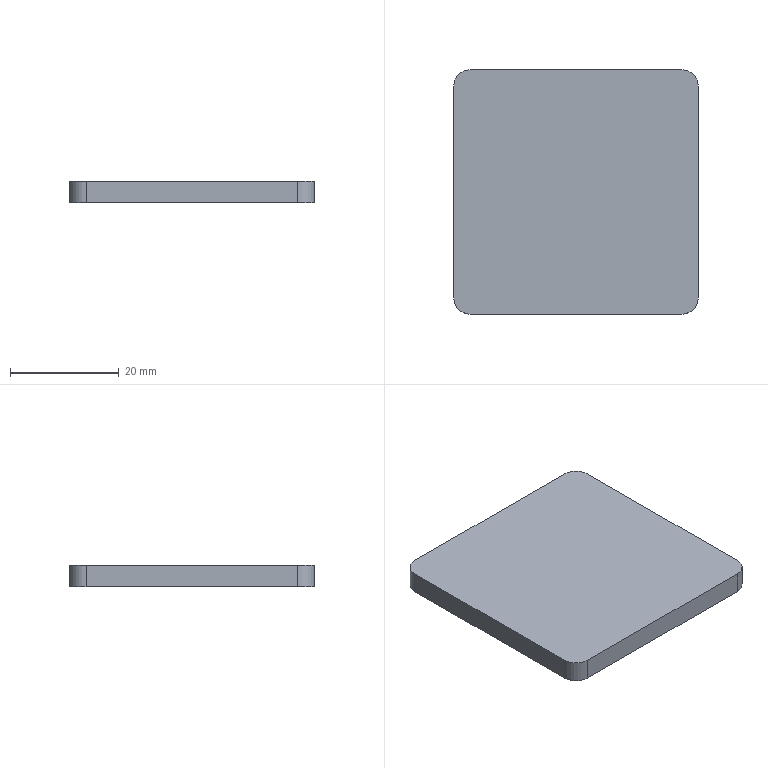Part | STEP file | 1 solid | 10 faces | box 45 x 45 x 4 mm | volume 8069 mm3 | plane 6 | cylinder 4 | commonest cylinder face diameters 6 x4
STEP:
#1=CARTESIAN_POINT('',(0.,0.,0.));
#2=DIRECTION('',(0.,0.,1.));
#3=DIRECTION('',(1.,0.,0.));
#4=AXIS2_PLACEMENT_3D('',#1,#2,#3);
#5=CARTESIAN_POINT('',(-527.5,-80.5,0.));
#6=VERTEX_POINT('',#5);
#7=CARTESIAN_POINT('',(-530.5,-77.5,0.));
#8=VERTEX_POINT('',#7);
#9=CARTESIAN_POINT('',(-530.5,-80.5,0.));
#10=DIRECTION('',(0.,0.,1.));
#11=DIRECTION('',(-1.,0.,0.));
#12=AXIS2_PLACEMENT_3D('',#9,#10,#11);
#13=CIRCLE('',#12,3.);
#14=CARTESIAN_POINT('',(-530.5,-80.5,0.));
#15=DIRECTION('',(0.,0.,-1.));
#16=DIRECTION('',(-1.,0.,0.));
#17=AXIS2_PLACEMENT_3D('',#14,#15,#16);
#18=PLANE('',#17);
#19=CARTESIAN_POINT('',(3.,0.));
#20=CARTESIAN_POINT('',(3.,-5.196));
#21=CARTESIAN_POINT('',(-1.5,-2.598));
#22=CARTESIAN_POINT('',(-6.,0.));
#23=CARTESIAN_POINT('',(-1.5,2.598));
#24=CARTESIAN_POINT('',(3.,5.196));
#25=CARTESIAN_POINT('',(3.,0.));
#26=(BOUNDED_CURVE()B_SPLINE_CURVE(2,(#19,#20,#21,#22,#23,#24,#25),.UNSPECIFIED.,.T.,.F.)B_SPLINE_CURVE_WITH_KNOTS((1,2,2,2,2,1),(-2.094,0.,2.094,4.189,6.283,8.378),.UNSPECIFIED.)CURVE()GEOMETRIC_REPRESENTATION_ITEM()RATIONAL_B_SPLINE_CURVE((1.,0.5,1.,0.5,1.,0.5,1.))REPRESENTATION_ITEM(''));
#27=(GEOMETRIC_REPRESENTATION_CONTEXT(2)PARAMETRIC_REPRESENTATION_CONTEXT()REPRESENTATION_CONTEXT('',''));
#28=DEFINITIONAL_REPRESENTATION('',(#26),#27);
#29=PCURVE('',#18,#28);
#30=CARTESIAN_POINT('',(-530.5,-80.5,4.));
#31=DIRECTION('',(0.,0.,-1.));
#32=DIRECTION('',(-1.,0.,0.));
#33=AXIS2_PLACEMENT_3D('',#30,#31,#32);
#34=CYLINDRICAL_SURFACE('',#33,3.);
#35=CARTESIAN_POINT('',(6.283,4.));
#36=DIRECTION('',(-1.,0.));
#37=VECTOR('',#36,1.);
#38=LINE('',#35,#37);
#39=(GEOMETRIC_REPRESENTATION_CONTEXT(2)PARAMETRIC_REPRESENTATION_CONTEXT()REPRESENTATION_CONTEXT('',''));
#40=DEFINITIONAL_REPRESENTATION('',(#38),#39);
#41=PCURVE('',#34,#40);
#42=SURFACE_CURVE('',#13,(#29,#41),.PCURVE_S1.);
#43=EDGE_CURVE('',#6,#8,#42,.T.);
#44=ORIENTED_EDGE('',*,*,#43,.F.);
#45=CARTESIAN_POINT('',(-527.5,-119.5,0.));
#46=VERTEX_POINT('',#45);
#47=CARTESIAN_POINT('',(-527.5,-80.5,0.));
#48=DIRECTION('',(0.,1.,0.));
#49=VECTOR('',#48,1.);
#50=LINE('',#47,#49);
#51=CARTESIAN_POINT('',(-3.,0.));
#52=DIRECTION('',(0.,1.));
#53=VECTOR('',#52,1.);
#54=LINE('',#51,#53);
#55=(GEOMETRIC_REPRESENTATION_CONTEXT(2)PARAMETRIC_REPRESENTATION_CONTEXT()REPRESENTATION_CONTEXT('',''));
#56=DEFINITIONAL_REPRESENTATION('',(#54),#55);
#57=PCURVE('',#18,#56);
#58=CARTESIAN_POINT('',(-527.5,-80.5,4.));
#59=DIRECTION('',(-1.,0.,0.));
#60=DIRECTION('',(0.,0.,1.));
#61=AXIS2_PLACEMENT_3D('',#58,#59,#60);
#62=PLANE('',#61);
#63=CARTESIAN_POINT('',(-4.,0.));
#64=DIRECTION('',(0.,1.));
#65=VECTOR('',#64,1.);
#66=LINE('',#63,#65);
#67=(GEOMETRIC_REPRESENTATION_CONTEXT(2)PARAMETRIC_REPRESENTATION_CONTEXT()REPRESENTATION_CONTEXT('',''));
#68=DEFINITIONAL_REPRESENTATION('',(#66),#67);
#69=PCURVE('',#62,#68);
#70=SURFACE_CURVE('',#50,(#57,#69),.PCURVE_S1.);
#71=EDGE_CURVE('',#46,#6,#70,.T.);
#72=ORIENTED_EDGE('',*,*,#71,.F.);
#73=CARTESIAN_POINT('',(-530.5,-122.5,0.));
#74=VERTEX_POINT('',#73);
#75=CARTESIAN_POINT('',(-530.5,-119.5,0.));
#76=DIRECTION('',(0.,0.,1.));
#77=DIRECTION('',(-1.,0.,0.));
#78=AXIS2_PLACEMENT_3D('',#75,#76,#77);
#79=CIRCLE('',#78,3.);
#80=CARTESIAN_POINT('',(3.,-39.));
#81=CARTESIAN_POINT('',(3.,-44.196));
#82=CARTESIAN_POINT('',(-1.5,-41.598));
#83=CARTESIAN_POINT('',(-6.,-39.));
#84=CARTESIAN_POINT('',(-1.5,-36.402));
#85=CARTESIAN_POINT('',(3.,-33.804));
#86=CARTESIAN_POINT('',(3.,-39.));
#87=(BOUNDED_CURVE()B_SPLINE_CURVE(2,(#80,#81,#82,#83,#84,#85,#86),.UNSPECIFIED.,.T.,.F.)B_SPLINE_CURVE_WITH_KNOTS((1,2,2,2,2,1),(-2.094,0.,2.094,4.189,6.283,8.378),.UNSPECIFIED.)CURVE()GEOMETRIC_REPRESENTATION_ITEM()RATIONAL_B_SPLINE_CURVE((1.,0.5,1.,0.5,1.,0.5,1.))REPRESENTATION_ITEM(''));
#88=(GEOMETRIC_REPRESENTATION_CONTEXT(2)PARAMETRIC_REPRESENTATION_CONTEXT()REPRESENTATION_CONTEXT('',''));
#89=DEFINITIONAL_REPRESENTATION('',(#87),#88);
#90=PCURVE('',#18,#89);
#91=CARTESIAN_POINT('',(-530.5,-119.5,4.));
#92=DIRECTION('',(0.,0.,-1.));
#93=DIRECTION('',(-1.,0.,0.));
#94=AXIS2_PLACEMENT_3D('',#91,#92,#93);
#95=CYLINDRICAL_SURFACE('',#94,3.);
#96=CARTESIAN_POINT('',(6.283,4.));
#97=DIRECTION('',(-1.,0.));
#98=VECTOR('',#97,1.);
#99=LINE('',#96,#98);
#100=(GEOMETRIC_REPRESENTATION_CONTEXT(2)PARAMETRIC_REPRESENTATION_CONTEXT()REPRESENTATION_CONTEXT('',''));
#101=DEFINITIONAL_REPRESENTATION('',(#99),#100);
#102=PCURVE('',#95,#101);
#103=SURFACE_CURVE('',#79,(#90,#102),.PCURVE_S1.);
#104=EDGE_CURVE('',#74,#46,#103,.T.);
#105=ORIENTED_EDGE('',*,*,#104,.F.);
#106=CARTESIAN_POINT('',(-569.5,-122.5,0.));
#107=VERTEX_POINT('',#106);
#108=CARTESIAN_POINT('',(-530.5,-122.5,0.));
#109=DIRECTION('',(1.,0.,0.));
#110=VECTOR('',#109,1.);
#111=LINE('',#108,#110);
#112=CARTESIAN_POINT('',(0.,-42.));
#113=DIRECTION('',(-1.,0.));
#114=VECTOR('',#113,1.);
#115=LINE('',#112,#114);
#116=(GEOMETRIC_REPRESENTATION_CONTEXT(2)PARAMETRIC_REPRESENTATION_CONTEXT()REPRESENTATION_CONTEXT('',''));
#117=DEFINITIONAL_REPRESENTATION('',(#115),#116);
#118=PCURVE('',#18,#117);
#119=CARTESIAN_POINT('',(-530.5,-122.5,4.));
#120=DIRECTION('',(0.,1.,0.));
#121=DIRECTION('',(1.,0.,0.));
#122=AXIS2_PLACEMENT_3D('',#119,#120,#121);
#123=PLANE('',#122);
#124=CARTESIAN_POINT('',(0.,4.));
#125=DIRECTION('',(1.,0.));
#126=VECTOR('',#125,1.);
#127=LINE('',#124,#126);
#128=(GEOMETRIC_REPRESENTATION_CONTEXT(2)PARAMETRIC_REPRESENTATION_CONTEXT()REPRESENTATION_CONTEXT('',''));
#129=DEFINITIONAL_REPRESENTATION('',(#127),#128);
#130=PCURVE('',#123,#129);
#131=SURFACE_CURVE('',#111,(#118,#130),.PCURVE_S1.);
#132=EDGE_CURVE('',#107,#74,#131,.T.);
#133=ORIENTED_EDGE('',*,*,#132,.F.);
#134=CARTESIAN_POINT('',(-572.5,-119.5,0.));
#135=VERTEX_POINT('',#134);
#136=CARTESIAN_POINT('',(-569.5,-119.5,0.));
#137=DIRECTION('',(0.,0.,1.));
#138=DIRECTION('',(-1.,0.,0.));
#139=AXIS2_PLACEMENT_3D('',#136,#137,#138);
#140=CIRCLE('',#139,3.);
#141=CARTESIAN_POINT('',(42.,-39.));
#142=CARTESIAN_POINT('',(42.,-44.196));
#143=CARTESIAN_POINT('',(37.5,-41.598));
#144=CARTESIAN_POINT('',(33.,-39.));
#145=CARTESIAN_POINT('',(37.5,-36.402));
#146=CARTESIAN_POINT('',(42.,-33.804));
#147=CARTESIAN_POINT('',(42.,-39.));
#148=(BOUNDED_CURVE()B_SPLINE_CURVE(2,(#141,#142,#143,#144,#145,#146,#147),.UNSPECIFIED.,.T.,.F.)B_SPLINE_CURVE_WITH_KNOTS((1,2,2,2,2,1),(-2.094,0.,2.094,4.189,6.283,8.378),.UNSPECIFIED.)CURVE()GEOMETRIC_REPRESENTATION_ITEM()RATIONAL_B_SPLINE_CURVE((1.,0.5,1.,0.5,1.,0.5,1.))REPRESENTATION_ITEM(''));
#149=(GEOMETRIC_REPRESENTATION_CONTEXT(2)PARAMETRIC_REPRESENTATION_CONTEXT()REPRESENTATION_CONTEXT('',''));
#150=DEFINITIONAL_REPRESENTATION('',(#148),#149);
#151=PCURVE('',#18,#150);
#152=CARTESIAN_POINT('',(-569.5,-119.5,4.));
#153=DIRECTION('',(0.,0.,-1.));
#154=DIRECTION('',(-1.,0.,0.));
#155=AXIS2_PLACEMENT_3D('',#152,#153,#154);
#156=CYLINDRICAL_SURFACE('',#155,3.);
#157=CARTESIAN_POINT('',(6.283,4.));
#158=DIRECTION('',(-1.,0.));
#159=VECTOR('',#158,1.);
#160=LINE('',#157,#159);
#161=(GEOMETRIC_REPRESENTATION_CONTEXT(2)PARAMETRIC_REPRESENTATION_CONTEXT()REPRESENTATION_CONTEXT('',''));
#162=DEFINITIONAL_REPRESENTATION('',(#160),#161);
#163=PCURVE('',#156,#162);
#164=SURFACE_CURVE('',#140,(#151,#163),.PCURVE_S1.);
#165=EDGE_CURVE('',#135,#107,#164,.T.);
#166=ORIENTED_EDGE('',*,*,#165,.F.);
#167=CARTESIAN_POINT('',(-572.5,-80.5,0.));
#168=VERTEX_POINT('',#167);
#169=CARTESIAN_POINT('',(-572.5,-80.5,0.));
#170=DIRECTION('',(0.,-1.,0.));
#171=VECTOR('',#170,1.);
#172=LINE('',#169,#171);
#173=CARTESIAN_POINT('',(42.,0.));
#174=DIRECTION('',(0.,-1.));
#175=VECTOR('',#174,1.);
#176=LINE('',#173,#175);
#177=(GEOMETRIC_REPRESENTATION_CONTEXT(2)PARAMETRIC_REPRESENTATION_CONTEXT()REPRESENTATION_CONTEXT('',''));
#178=DEFINITIONAL_REPRESENTATION('',(#176),#177);
#179=PCURVE('',#18,#178);
#180=CARTESIAN_POINT('',(-572.5,-80.5,4.));
#181=DIRECTION('',(1.,0.,0.));
#182=DIRECTION('',(0.,0.,1.));
#183=AXIS2_PLACEMENT_3D('',#180,#181,#182);
#184=PLANE('',#183);
#185=CARTESIAN_POINT('',(-4.,0.));
#186=DIRECTION('',(0.,1.));
#187=VECTOR('',#186,1.);
#188=LINE('',#185,#187);
#189=(GEOMETRIC_REPRESENTATION_CONTEXT(2)PARAMETRIC_REPRESENTATION_CONTEXT()REPRESENTATION_CONTEXT('',''));
#190=DEFINITIONAL_REPRESENTATION('',(#188),#189);
#191=PCURVE('',#184,#190);
#192=SURFACE_CURVE('',#172,(#179,#191),.PCURVE_S1.);
#193=EDGE_CURVE('',#168,#135,#192,.T.);
#194=ORIENTED_EDGE('',*,*,#193,.F.);
#195=CARTESIAN_POINT('',(-569.5,-77.5,0.));
#196=VERTEX_POINT('',#195);
#197=CARTESIAN_POINT('',(-569.5,-80.5,0.));
#198=DIRECTION('',(0.,0.,1.));
#199=DIRECTION('',(1.,0.,0.));
#200=AXIS2_PLACEMENT_3D('',#197,#198,#199);
#201=CIRCLE('',#200,3.);
#202=CARTESIAN_POINT('',(36.,0.));
#203=CARTESIAN_POINT('',(36.,5.196));
#204=CARTESIAN_POINT('',(40.5,2.598));
#205=CARTESIAN_POINT('',(45.,0.));
#206=CARTESIAN_POINT('',(40.5,-2.598));
#207=CARTESIAN_POINT('',(36.,-5.196));
#208=CARTESIAN_POINT('',(36.,0.));
#209=(BOUNDED_CURVE()B_SPLINE_CURVE(2,(#202,#203,#204,#205,#206,#207,#208),.UNSPECIFIED.,.T.,.F.)B_SPLINE_CURVE_WITH_KNOTS((1,2,2,2,2,1),(-2.094,0.,2.094,4.189,6.283,8.378),.UNSPECIFIED.)CURVE()GEOMETRIC_REPRESENTATION_ITEM()RATIONAL_B_SPLINE_CURVE((1.,0.5,1.,0.5,1.,0.5,1.))REPRESENTATION_ITEM(''));
#210=(GEOMETRIC_REPRESENTATION_CONTEXT(2)PARAMETRIC_REPRESENTATION_CONTEXT()REPRESENTATION_CONTEXT('',''));
#211=DEFINITIONAL_REPRESENTATION('',(#209),#210);
#212=PCURVE('',#18,#211);
#213=CARTESIAN_POINT('',(-569.5,-80.5,4.));
#214=DIRECTION('',(0.,0.,-1.));
#215=DIRECTION('',(-1.,0.,0.));
#216=AXIS2_PLACEMENT_3D('',#213,#214,#215);
#217=CYLINDRICAL_SURFACE('',#216,3.);
#218=CARTESIAN_POINT('',(3.142,4.));
#219=DIRECTION('',(-1.,0.));
#220=VECTOR('',#219,1.);
#221=LINE('',#218,#220);
#222=(GEOMETRIC_REPRESENTATION_CONTEXT(2)PARAMETRIC_REPRESENTATION_CONTEXT()REPRESENTATION_CONTEXT('',''));
#223=DEFINITIONAL_REPRESENTATION('',(#221),#222);
#224=PCURVE('',#217,#223);
#225=SURFACE_CURVE('',#201,(#212,#224),.PCURVE_S1.);
#226=EDGE_CURVE('',#196,#168,#225,.T.);
#227=ORIENTED_EDGE('',*,*,#226,.F.);
#228=CARTESIAN_POINT('',(-530.5,-77.5,0.));
#229=DIRECTION('',(-1.,0.,0.));
#230=VECTOR('',#229,1.);
#231=LINE('',#228,#230);
#232=CARTESIAN_POINT('',(0.,3.));
#233=DIRECTION('',(1.,0.));
#234=VECTOR('',#233,1.);
#235=LINE('',#232,#234);
#236=(GEOMETRIC_REPRESENTATION_CONTEXT(2)PARAMETRIC_REPRESENTATION_CONTEXT()REPRESENTATION_CONTEXT('',''));
#237=DEFINITIONAL_REPRESENTATION('',(#235),#236);
#238=PCURVE('',#18,#237);
#239=CARTESIAN_POINT('',(-530.5,-77.5,4.));
#240=DIRECTION('',(0.,-1.,0.));
#241=DIRECTION('',(0.,0.,-1.));
#242=AXIS2_PLACEMENT_3D('',#239,#240,#241);
#243=PLANE('',#242);
#244=CARTESIAN_POINT('',(4.,0.));
#245=DIRECTION('',(0.,-1.));
#246=VECTOR('',#245,1.);
#247=LINE('',#244,#246);
#248=(GEOMETRIC_REPRESENTATION_CONTEXT(2)PARAMETRIC_REPRESENTATION_CONTEXT()REPRESENTATION_CONTEXT('',''));
#249=DEFINITIONAL_REPRESENTATION('',(#247),#248);
#250=PCURVE('',#243,#249);
#251=SURFACE_CURVE('',#231,(#238,#250),.PCURVE_S1.);
#252=EDGE_CURVE('',#8,#196,#251,.T.);
#253=ORIENTED_EDGE('',*,*,#252,.F.);
#254=EDGE_LOOP('',(#44,#72,#105,#133,#166,#194,#227,#253));
#255=FACE_BOUND('',#254,.T.);
#256=ADVANCED_FACE('',(#255),#18,.T.);
#257=CARTESIAN_POINT('',(-527.5,-80.5,4.));
#258=VERTEX_POINT('',#257);
#259=CARTESIAN_POINT('',(-530.5,-77.5,4.));
#260=VERTEX_POINT('',#259);
#261=CARTESIAN_POINT('',(-530.5,-80.5,4.));
#262=DIRECTION('',(0.,0.,1.));
#263=DIRECTION('',(-1.,0.,0.));
#264=AXIS2_PLACEMENT_3D('',#261,#262,#263);
#265=CIRCLE('',#264,3.);
#266=CARTESIAN_POINT('',(-530.5,-80.5,4.));
#267=DIRECTION('',(0.,0.,-1.));
#268=DIRECTION('',(-1.,0.,0.));
#269=AXIS2_PLACEMENT_3D('',#266,#267,#268);
#270=PLANE('',#269);
#271=CARTESIAN_POINT('',(3.,0.));
#272=CARTESIAN_POINT('',(3.,-5.196));
#273=CARTESIAN_POINT('',(-1.5,-2.598));
#274=CARTESIAN_POINT('',(-6.,0.));
#275=CARTESIAN_POINT('',(-1.5,2.598));
#276=CARTESIAN_POINT('',(3.,5.196));
#277=CARTESIAN_POINT('',(3.,0.));
#278=(BOUNDED_CURVE()B_SPLINE_CURVE(2,(#271,#272,#273,#274,#275,#276,#277),.UNSPECIFIED.,.T.,.F.)B_SPLINE_CURVE_WITH_KNOTS((1,2,2,2,2,1),(-2.094,0.,2.094,4.189,6.283,8.378),.UNSPECIFIED.)CURVE()GEOMETRIC_REPRESENTATION_ITEM()RATIONAL_B_SPLINE_CURVE((1.,0.5,1.,0.5,1.,0.5,1.))REPRESENTATION_ITEM(''));
#279=(GEOMETRIC_REPRESENTATION_CONTEXT(2)PARAMETRIC_REPRESENTATION_CONTEXT()REPRESENTATION_CONTEXT('',''));
#280=DEFINITIONAL_REPRESENTATION('',(#278),#279);
#281=PCURVE('',#270,#280);
#282=CARTESIAN_POINT('',(6.283,0.));
#283=DIRECTION('',(-1.,0.));
#284=VECTOR('',#283,1.);
#285=LINE('',#282,#284);
#286=(GEOMETRIC_REPRESENTATION_CONTEXT(2)PARAMETRIC_REPRESENTATION_CONTEXT()REPRESENTATION_CONTEXT('',''));
#287=DEFINITIONAL_REPRESENTATION('',(#285),#286);
#288=PCURVE('',#34,#287);
#289=SURFACE_CURVE('',#265,(#281,#288),.PCURVE_S1.);
#290=EDGE_CURVE('',#258,#260,#289,.T.);
#291=ORIENTED_EDGE('',*,*,#290,.T.);
#292=CARTESIAN_POINT('',(-569.5,-77.5,4.));
#293=VERTEX_POINT('',#292);
#294=CARTESIAN_POINT('',(-530.5,-77.5,4.));
#295=DIRECTION('',(-1.,0.,0.));
#296=VECTOR('',#295,1.);
#297=LINE('',#294,#296);
#298=CARTESIAN_POINT('',(0.,3.));
#299=DIRECTION('',(1.,0.));
#300=VECTOR('',#299,1.);
#301=LINE('',#298,#300);
#302=(GEOMETRIC_REPRESENTATION_CONTEXT(2)PARAMETRIC_REPRESENTATION_CONTEXT()REPRESENTATION_CONTEXT('',''));
#303=DEFINITIONAL_REPRESENTATION('',(#301),#302);
#304=PCURVE('',#270,#303);
#305=CARTESIAN_POINT('',(0.,0.));
#306=DIRECTION('',(0.,-1.));
#307=VECTOR('',#306,1.);
#308=LINE('',#305,#307);
#309=(GEOMETRIC_REPRESENTATION_CONTEXT(2)PARAMETRIC_REPRESENTATION_CONTEXT()REPRESENTATION_CONTEXT('',''));
#310=DEFINITIONAL_REPRESENTATION('',(#308),#309);
#311=PCURVE('',#243,#310);
#312=SURFACE_CURVE('',#297,(#304,#311),.PCURVE_S1.);
#313=EDGE_CURVE('',#260,#293,#312,.T.);
#314=ORIENTED_EDGE('',*,*,#313,.T.);
#315=CARTESIAN_POINT('',(-572.5,-80.5,4.));
#316=VERTEX_POINT('',#315);
#317=CARTESIAN_POINT('',(-569.5,-80.5,4.));
#318=DIRECTION('',(0.,0.,1.));
#319=DIRECTION('',(1.,0.,0.));
#320=AXIS2_PLACEMENT_3D('',#317,#318,#319);
#321=CIRCLE('',#320,3.);
#322=CARTESIAN_POINT('',(36.,0.));
#323=CARTESIAN_POINT('',(36.,5.196));
#324=CARTESIAN_POINT('',(40.5,2.598));
#325=CARTESIAN_POINT('',(45.,0.));
#326=CARTESIAN_POINT('',(40.5,-2.598));
#327=CARTESIAN_POINT('',(36.,-5.196));
#328=CARTESIAN_POINT('',(36.,0.));
#329=(BOUNDED_CURVE()B_SPLINE_CURVE(2,(#322,#323,#324,#325,#326,#327,#328),.UNSPECIFIED.,.T.,.F.)B_SPLINE_CURVE_WITH_KNOTS((1,2,2,2,2,1),(-2.094,0.,2.094,4.189,6.283,8.378),.UNSPECIFIED.)CURVE()GEOMETRIC_REPRESENTATION_ITEM()RATIONAL_B_SPLINE_CURVE((1.,0.5,1.,0.5,1.,0.5,1.))REPRESENTATION_ITEM(''));
#330=(GEOMETRIC_REPRESENTATION_CONTEXT(2)PARAMETRIC_REPRESENTATION_CONTEXT()REPRESENTATION_CONTEXT('',''));
#331=DEFINITIONAL_REPRESENTATION('',(#329),#330);
#332=PCURVE('',#270,#331);
#333=CARTESIAN_POINT('',(3.142,0.));
#334=DIRECTION('',(-1.,0.));
#335=VECTOR('',#334,1.);
#336=LINE('',#333,#335);
#337=(GEOMETRIC_REPRESENTATION_CONTEXT(2)PARAMETRIC_REPRESENTATION_CONTEXT()REPRESENTATION_CONTEXT('',''));
#338=DEFINITIONAL_REPRESENTATION('',(#336),#337);
#339=PCURVE('',#217,#338);
#340=SURFACE_CURVE('',#321,(#332,#339),.PCURVE_S1.);
#341=EDGE_CURVE('',#293,#316,#340,.T.);
#342=ORIENTED_EDGE('',*,*,#341,.T.);
#343=CARTESIAN_POINT('',(-572.5,-119.5,4.));
#344=VERTEX_POINT('',#343);
#345=CARTESIAN_POINT('',(-572.5,-80.5,4.));
#346=DIRECTION('',(0.,-1.,0.));
#347=VECTOR('',#346,1.);
#348=LINE('',#345,#347);
#349=CARTESIAN_POINT('',(42.,0.));
#350=DIRECTION('',(0.,-1.));
#351=VECTOR('',#350,1.);
#352=LINE('',#349,#351);
#353=(GEOMETRIC_REPRESENTATION_CONTEXT(2)PARAMETRIC_REPRESENTATION_CONTEXT()REPRESENTATION_CONTEXT('',''));
#354=DEFINITIONAL_REPRESENTATION('',(#352),#353);
#355=PCURVE('',#270,#354);
#356=CARTESIAN_POINT('',(0.,0.));
#357=DIRECTION('',(0.,1.));
#358=VECTOR('',#357,1.);
#359=LINE('',#356,#358);
#360=(GEOMETRIC_REPRESENTATION_CONTEXT(2)PARAMETRIC_REPRESENTATION_CONTEXT()REPRESENTATION_CONTEXT('',''));
#361=DEFINITIONAL_REPRESENTATION('',(#359),#360);
#362=PCURVE('',#184,#361);
#363=SURFACE_CURVE('',#348,(#355,#362),.PCURVE_S1.);
#364=EDGE_CURVE('',#316,#344,#363,.T.);
#365=ORIENTED_EDGE('',*,*,#364,.T.);
#366=CARTESIAN_POINT('',(-569.5,-122.5,4.));
#367=VERTEX_POINT('',#366);
#368=CARTESIAN_POINT('',(-569.5,-119.5,4.));
#369=DIRECTION('',(0.,0.,1.));
#370=DIRECTION('',(-1.,0.,0.));
#371=AXIS2_PLACEMENT_3D('',#368,#369,#370);
#372=CIRCLE('',#371,3.);
#373=CARTESIAN_POINT('',(42.,-39.));
#374=CARTESIAN_POINT('',(42.,-44.196));
#375=CARTESIAN_POINT('',(37.5,-41.598));
#376=CARTESIAN_POINT('',(33.,-39.));
#377=CARTESIAN_POINT('',(37.5,-36.402));
#378=CARTESIAN_POINT('',(42.,-33.804));
#379=CARTESIAN_POINT('',(42.,-39.));
#380=(BOUNDED_CURVE()B_SPLINE_CURVE(2,(#373,#374,#375,#376,#377,#378,#379),.UNSPECIFIED.,.T.,.F.)B_SPLINE_CURVE_WITH_KNOTS((1,2,2,2,2,1),(-2.094,0.,2.094,4.189,6.283,8.378),.UNSPECIFIED.)CURVE()GEOMETRIC_REPRESENTATION_ITEM()RATIONAL_B_SPLINE_CURVE((1.,0.5,1.,0.5,1.,0.5,1.))REPRESENTATION_ITEM(''));
#381=(GEOMETRIC_REPRESENTATION_CONTEXT(2)PARAMETRIC_REPRESENTATION_CONTEXT()REPRESENTATION_CONTEXT('',''));
#382=DEFINITIONAL_REPRESENTATION('',(#380),#381);
#383=PCURVE('',#270,#382);
#384=CARTESIAN_POINT('',(6.283,0.));
#385=DIRECTION('',(-1.,0.));
#386=VECTOR('',#385,1.);
#387=LINE('',#384,#386);
#388=(GEOMETRIC_REPRESENTATION_CONTEXT(2)PARAMETRIC_REPRESENTATION_CONTEXT()REPRESENTATION_CONTEXT('',''));
#389=DEFINITIONAL_REPRESENTATION('',(#387),#388);
#390=PCURVE('',#156,#389);
#391=SURFACE_CURVE('',#372,(#383,#390),.PCURVE_S1.);
#392=EDGE_CURVE('',#344,#367,#391,.T.);
#393=ORIENTED_EDGE('',*,*,#392,.T.);
#394=CARTESIAN_POINT('',(-530.5,-122.5,4.));
#395=VERTEX_POINT('',#394);
#396=CARTESIAN_POINT('',(-530.5,-122.5,4.));
#397=DIRECTION('',(1.,0.,0.));
#398=VECTOR('',#397,1.);
#399=LINE('',#396,#398);
#400=CARTESIAN_POINT('',(0.,-42.));
#401=DIRECTION('',(-1.,0.));
#402=VECTOR('',#401,1.);
#403=LINE('',#400,#402);
#404=(GEOMETRIC_REPRESENTATION_CONTEXT(2)PARAMETRIC_REPRESENTATION_CONTEXT()REPRESENTATION_CONTEXT('',''));
#405=DEFINITIONAL_REPRESENTATION('',(#403),#404);
#406=PCURVE('',#270,#405);
#407=CARTESIAN_POINT('',(0.,0.));
#408=DIRECTION('',(1.,0.));
#409=VECTOR('',#408,1.);
#410=LINE('',#407,#409);
#411=(GEOMETRIC_REPRESENTATION_CONTEXT(2)PARAMETRIC_REPRESENTATION_CONTEXT()REPRESENTATION_CONTEXT('',''));
#412=DEFINITIONAL_REPRESENTATION('',(#410),#411);
#413=PCURVE('',#123,#412);
#414=SURFACE_CURVE('',#399,(#406,#413),.PCURVE_S1.);
#415=EDGE_CURVE('',#367,#395,#414,.T.);
#416=ORIENTED_EDGE('',*,*,#415,.T.);
#417=CARTESIAN_POINT('',(-527.5,-119.5,4.));
#418=VERTEX_POINT('',#417);
#419=CARTESIAN_POINT('',(-530.5,-119.5,4.));
#420=DIRECTION('',(0.,0.,1.));
#421=DIRECTION('',(-1.,0.,0.));
#422=AXIS2_PLACEMENT_3D('',#419,#420,#421);
#423=CIRCLE('',#422,3.);
#424=CARTESIAN_POINT('',(3.,-39.));
#425=CARTESIAN_POINT('',(3.,-44.196));
#426=CARTESIAN_POINT('',(-1.5,-41.598));
#427=CARTESIAN_POINT('',(-6.,-39.));
#428=CARTESIAN_POINT('',(-1.5,-36.402));
#429=CARTESIAN_POINT('',(3.,-33.804));
#430=CARTESIAN_POINT('',(3.,-39.));
#431=(BOUNDED_CURVE()B_SPLINE_CURVE(2,(#424,#425,#426,#427,#428,#429,#430),.UNSPECIFIED.,.T.,.F.)B_SPLINE_CURVE_WITH_KNOTS((1,2,2,2,2,1),(-2.094,0.,2.094,4.189,6.283,8.378),.UNSPECIFIED.)CURVE()GEOMETRIC_REPRESENTATION_ITEM()RATIONAL_B_SPLINE_CURVE((1.,0.5,1.,0.5,1.,0.5,1.))REPRESENTATION_ITEM(''));
#432=(GEOMETRIC_REPRESENTATION_CONTEXT(2)PARAMETRIC_REPRESENTATION_CONTEXT()REPRESENTATION_CONTEXT('',''));
#433=DEFINITIONAL_REPRESENTATION('',(#431),#432);
#434=PCURVE('',#270,#433);
#435=CARTESIAN_POINT('',(6.283,0.));
#436=DIRECTION('',(-1.,0.));
#437=VECTOR('',#436,1.);
#438=LINE('',#435,#437);
#439=(GEOMETRIC_REPRESENTATION_CONTEXT(2)PARAMETRIC_REPRESENTATION_CONTEXT()REPRESENTATION_CONTEXT('',''));
#440=DEFINITIONAL_REPRESENTATION('',(#438),#439);
#441=PCURVE('',#95,#440);
#442=SURFACE_CURVE('',#423,(#434,#441),.PCURVE_S1.);
#443=EDGE_CURVE('',#395,#418,#442,.T.);
#444=ORIENTED_EDGE('',*,*,#443,.T.);
#445=CARTESIAN_POINT('',(-527.5,-80.5,4.));
#446=DIRECTION('',(0.,1.,0.));
#447=VECTOR('',#446,1.);
#448=LINE('',#445,#447);
#449=CARTESIAN_POINT('',(-3.,0.));
#450=DIRECTION('',(0.,1.));
#451=VECTOR('',#450,1.);
#452=LINE('',#449,#451);
#453=(GEOMETRIC_REPRESENTATION_CONTEXT(2)PARAMETRIC_REPRESENTATION_CONTEXT()REPRESENTATION_CONTEXT('',''));
#454=DEFINITIONAL_REPRESENTATION('',(#452),#453);
#455=PCURVE('',#270,#454);
#456=CARTESIAN_POINT('',(0.,0.));
#457=DIRECTION('',(0.,1.));
#458=VECTOR('',#457,1.);
#459=LINE('',#456,#458);
#460=(GEOMETRIC_REPRESENTATION_CONTEXT(2)PARAMETRIC_REPRESENTATION_CONTEXT()REPRESENTATION_CONTEXT('',''));
#461=DEFINITIONAL_REPRESENTATION('',(#459),#460);
#462=PCURVE('',#62,#461);
#463=SURFACE_CURVE('',#448,(#455,#462),.PCURVE_S1.);
#464=EDGE_CURVE('',#418,#258,#463,.T.);
#465=ORIENTED_EDGE('',*,*,#464,.T.);
#466=EDGE_LOOP('',(#291,#314,#342,#365,#393,#416,#444,#465));
#467=FACE_BOUND('',#466,.T.);
#468=ADVANCED_FACE('',(#467),#270,.F.);
#469=ORIENTED_EDGE('',*,*,#71,.T.);
#470=CARTESIAN_POINT('',(-527.5,-80.5,4.));
#471=DIRECTION('',(0.,0.,-1.));
#472=VECTOR('',#471,1.);
#473=LINE('',#470,#472);
#474=CARTESIAN_POINT('',(0.,0.));
#475=DIRECTION('',(-1.,0.));
#476=VECTOR('',#475,1.);
#477=LINE('',#474,#476);
#478=(GEOMETRIC_REPRESENTATION_CONTEXT(2)PARAMETRIC_REPRESENTATION_CONTEXT()REPRESENTATION_CONTEXT('',''));
#479=DEFINITIONAL_REPRESENTATION('',(#477),#478);
#480=PCURVE('',#62,#479);
#481=CARTESIAN_POINT('',(3.142,0.));
#482=DIRECTION('',(0.,1.));
#483=VECTOR('',#482,1.);
#484=LINE('',#481,#483);
#485=(GEOMETRIC_REPRESENTATION_CONTEXT(2)PARAMETRIC_REPRESENTATION_CONTEXT()REPRESENTATION_CONTEXT('',''));
#486=DEFINITIONAL_REPRESENTATION('',(#484),#485);
#487=PCURVE('',#34,#486);
#488=SURFACE_CURVE('',#473,(#480,#487),.PCURVE_S1.);
#489=EDGE_CURVE('',#258,#6,#488,.T.);
#490=ORIENTED_EDGE('',*,*,#489,.F.);
#491=ORIENTED_EDGE('',*,*,#464,.F.);
#492=CARTESIAN_POINT('',(-527.5,-119.5,4.));
#493=DIRECTION('',(0.,0.,-1.));
#494=VECTOR('',#493,1.);
#495=LINE('',#492,#494);
#496=CARTESIAN_POINT('',(0.,-39.));
#497=DIRECTION('',(-1.,0.));
#498=VECTOR('',#497,1.);
#499=LINE('',#496,#498);
#500=(GEOMETRIC_REPRESENTATION_CONTEXT(2)PARAMETRIC_REPRESENTATION_CONTEXT()REPRESENTATION_CONTEXT('',''));
#501=DEFINITIONAL_REPRESENTATION('',(#499),#500);
#502=PCURVE('',#62,#501);
#503=CARTESIAN_POINT('',(3.142,0.));
#504=DIRECTION('',(0.,1.));
#505=VECTOR('',#504,1.);
#506=LINE('',#503,#505);
#507=(GEOMETRIC_REPRESENTATION_CONTEXT(2)PARAMETRIC_REPRESENTATION_CONTEXT()REPRESENTATION_CONTEXT('',''));
#508=DEFINITIONAL_REPRESENTATION('',(#506),#507);
#509=PCURVE('',#95,#508);
#510=SURFACE_CURVE('',#495,(#502,#509),.PCURVE_S1.);
#511=EDGE_CURVE('',#418,#46,#510,.T.);
#512=ORIENTED_EDGE('',*,*,#511,.T.);
#513=EDGE_LOOP('',(#469,#490,#491,#512));
#514=FACE_BOUND('',#513,.T.);
#515=ADVANCED_FACE('',(#514),#62,.F.);
#516=ORIENTED_EDGE('',*,*,#104,.T.);
#517=ORIENTED_EDGE('',*,*,#511,.F.);
#518=ORIENTED_EDGE('',*,*,#443,.F.);
#519=CARTESIAN_POINT('',(-530.5,-122.5,4.));
#520=DIRECTION('',(0.,0.,-1.));
#521=VECTOR('',#520,1.);
#522=LINE('',#519,#521);
#523=CARTESIAN_POINT('',(4.712,0.));
#524=DIRECTION('',(0.,1.));
#525=VECTOR('',#524,1.);
#526=LINE('',#523,#525);
#527=(GEOMETRIC_REPRESENTATION_CONTEXT(2)PARAMETRIC_REPRESENTATION_CONTEXT()REPRESENTATION_CONTEXT('',''));
#528=DEFINITIONAL_REPRESENTATION('',(#526),#527);
#529=PCURVE('',#95,#528);
#530=CARTESIAN_POINT('',(0.,0.));
#531=DIRECTION('',(0.,1.));
#532=VECTOR('',#531,1.);
#533=LINE('',#530,#532);
#534=(GEOMETRIC_REPRESENTATION_CONTEXT(2)PARAMETRIC_REPRESENTATION_CONTEXT()REPRESENTATION_CONTEXT('',''));
#535=DEFINITIONAL_REPRESENTATION('',(#533),#534);
#536=PCURVE('',#123,#535);
#537=SURFACE_CURVE('',#522,(#529,#536),.PCURVE_S1.);
#538=EDGE_CURVE('',#395,#74,#537,.T.);
#539=ORIENTED_EDGE('',*,*,#538,.T.);
#540=EDGE_LOOP('',(#516,#517,#518,#539));
#541=FACE_BOUND('',#540,.T.);
#542=ADVANCED_FACE('',(#541),#95,.T.);
#543=ORIENTED_EDGE('',*,*,#132,.T.);
#544=ORIENTED_EDGE('',*,*,#538,.F.);
#545=ORIENTED_EDGE('',*,*,#415,.F.);
#546=CARTESIAN_POINT('',(-569.5,-122.5,4.));
#547=DIRECTION('',(0.,0.,-1.));
#548=VECTOR('',#547,1.);
#549=LINE('',#546,#548);
#550=CARTESIAN_POINT('',(-39.,0.));
#551=DIRECTION('',(0.,1.));
#552=VECTOR('',#551,1.);
#553=LINE('',#550,#552);
#554=(GEOMETRIC_REPRESENTATION_CONTEXT(2)PARAMETRIC_REPRESENTATION_CONTEXT()REPRESENTATION_CONTEXT('',''));
#555=DEFINITIONAL_REPRESENTATION('',(#553),#554);
#556=PCURVE('',#123,#555);
#557=CARTESIAN_POINT('',(4.712,0.));
#558=DIRECTION('',(0.,1.));
#559=VECTOR('',#558,1.);
#560=LINE('',#557,#559);
#561=(GEOMETRIC_REPRESENTATION_CONTEXT(2)PARAMETRIC_REPRESENTATION_CONTEXT()REPRESENTATION_CONTEXT('',''));
#562=DEFINITIONAL_REPRESENTATION('',(#560),#561);
#563=PCURVE('',#156,#562);
#564=SURFACE_CURVE('',#549,(#556,#563),.PCURVE_S1.);
#565=EDGE_CURVE('',#367,#107,#564,.T.);
#566=ORIENTED_EDGE('',*,*,#565,.T.);
#567=EDGE_LOOP('',(#543,#544,#545,#566));
#568=FACE_BOUND('',#567,.T.);
#569=ADVANCED_FACE('',(#568),#123,.F.);
#570=ORIENTED_EDGE('',*,*,#165,.T.);
#571=ORIENTED_EDGE('',*,*,#565,.F.);
#572=ORIENTED_EDGE('',*,*,#392,.F.);
#573=CARTESIAN_POINT('',(-572.5,-119.5,4.));
#574=DIRECTION('',(0.,0.,-1.));
#575=VECTOR('',#574,1.);
#576=LINE('',#573,#575);
#577=CARTESIAN_POINT('',(6.283,0.));
#578=DIRECTION('',(0.,1.));
#579=VECTOR('',#578,1.);
#580=LINE('',#577,#579);
#581=(GEOMETRIC_REPRESENTATION_CONTEXT(2)PARAMETRIC_REPRESENTATION_CONTEXT()REPRESENTATION_CONTEXT('',''));
#582=DEFINITIONAL_REPRESENTATION('',(#580),#581);
#583=PCURVE('',#156,#582);
#584=CARTESIAN_POINT('',(0.,39.));
#585=DIRECTION('',(-1.,0.));
#586=VECTOR('',#585,1.);
#587=LINE('',#584,#586);
#588=(GEOMETRIC_REPRESENTATION_CONTEXT(2)PARAMETRIC_REPRESENTATION_CONTEXT()REPRESENTATION_CONTEXT('',''));
#589=DEFINITIONAL_REPRESENTATION('',(#587),#588);
#590=PCURVE('',#184,#589);
#591=SURFACE_CURVE('',#576,(#583,#590),.PCURVE_S1.);
#592=EDGE_CURVE('',#344,#135,#591,.T.);
#593=ORIENTED_EDGE('',*,*,#592,.T.);
#594=EDGE_LOOP('',(#570,#571,#572,#593));
#595=FACE_BOUND('',#594,.T.);
#596=ADVANCED_FACE('',(#595),#156,.T.);
#597=ORIENTED_EDGE('',*,*,#193,.T.);
#598=ORIENTED_EDGE('',*,*,#592,.F.);
#599=ORIENTED_EDGE('',*,*,#364,.F.);
#600=CARTESIAN_POINT('',(-572.5,-80.5,4.));
#601=DIRECTION('',(0.,0.,-1.));
#602=VECTOR('',#601,1.);
#603=LINE('',#600,#602);
#604=CARTESIAN_POINT('',(0.,0.));
#605=DIRECTION('',(-1.,0.));
#606=VECTOR('',#605,1.);
#607=LINE('',#604,#606);
#608=(GEOMETRIC_REPRESENTATION_CONTEXT(2)PARAMETRIC_REPRESENTATION_CONTEXT()REPRESENTATION_CONTEXT('',''));
#609=DEFINITIONAL_REPRESENTATION('',(#607),#608);
#610=PCURVE('',#184,#609);
#611=CARTESIAN_POINT('',(0.,0.));
#612=DIRECTION('',(0.,1.));
#613=VECTOR('',#612,1.);
#614=LINE('',#611,#613);
#615=(GEOMETRIC_REPRESENTATION_CONTEXT(2)PARAMETRIC_REPRESENTATION_CONTEXT()REPRESENTATION_CONTEXT('',''));
#616=DEFINITIONAL_REPRESENTATION('',(#614),#615);
#617=PCURVE('',#217,#616);
#618=SURFACE_CURVE('',#603,(#610,#617),.PCURVE_S1.);
#619=EDGE_CURVE('',#316,#168,#618,.T.);
#620=ORIENTED_EDGE('',*,*,#619,.T.);
#621=EDGE_LOOP('',(#597,#598,#599,#620));
#622=FACE_BOUND('',#621,.T.);
#623=ADVANCED_FACE('',(#622),#184,.F.);
#624=ORIENTED_EDGE('',*,*,#226,.T.);
#625=ORIENTED_EDGE('',*,*,#619,.F.);
#626=ORIENTED_EDGE('',*,*,#341,.F.);
#627=CARTESIAN_POINT('',(-569.5,-77.5,4.));
#628=DIRECTION('',(0.,0.,-1.));
#629=VECTOR('',#628,1.);
#630=LINE('',#627,#629);
#631=CARTESIAN_POINT('',(1.571,0.));
#632=DIRECTION('',(0.,1.));
#633=VECTOR('',#632,1.);
#634=LINE('',#631,#633);
#635=(GEOMETRIC_REPRESENTATION_CONTEXT(2)PARAMETRIC_REPRESENTATION_CONTEXT()REPRESENTATION_CONTEXT('',''));
#636=DEFINITIONAL_REPRESENTATION('',(#634),#635);
#637=PCURVE('',#217,#636);
#638=CARTESIAN_POINT('',(0.,-39.));
#639=DIRECTION('',(1.,0.));
#640=VECTOR('',#639,1.);
#641=LINE('',#638,#640);
#642=(GEOMETRIC_REPRESENTATION_CONTEXT(2)PARAMETRIC_REPRESENTATION_CONTEXT()REPRESENTATION_CONTEXT('',''));
#643=DEFINITIONAL_REPRESENTATION('',(#641),#642);
#644=PCURVE('',#243,#643);
#645=SURFACE_CURVE('',#630,(#637,#644),.PCURVE_S1.);
#646=EDGE_CURVE('',#293,#196,#645,.T.);
#647=ORIENTED_EDGE('',*,*,#646,.T.);
#648=EDGE_LOOP('',(#624,#625,#626,#647));
#649=FACE_BOUND('',#648,.T.);
#650=ADVANCED_FACE('',(#649),#217,.T.);
#651=ORIENTED_EDGE('',*,*,#252,.T.);
#652=ORIENTED_EDGE('',*,*,#646,.F.);
#653=ORIENTED_EDGE('',*,*,#313,.F.);
#654=CARTESIAN_POINT('',(-530.5,-77.5,4.));
#655=DIRECTION('',(0.,0.,-1.));
#656=VECTOR('',#655,1.);
#657=LINE('',#654,#656);
#658=CARTESIAN_POINT('',(0.,0.));
#659=DIRECTION('',(1.,0.));
#660=VECTOR('',#659,1.);
#661=LINE('',#658,#660);
#662=(GEOMETRIC_REPRESENTATION_CONTEXT(2)PARAMETRIC_REPRESENTATION_CONTEXT()REPRESENTATION_CONTEXT('',''));
#663=DEFINITIONAL_REPRESENTATION('',(#661),#662);
#664=PCURVE('',#243,#663);
#665=CARTESIAN_POINT('',(1.571,0.));
#666=DIRECTION('',(0.,1.));
#667=VECTOR('',#666,1.);
#668=LINE('',#665,#667);
#669=(GEOMETRIC_REPRESENTATION_CONTEXT(2)PARAMETRIC_REPRESENTATION_CONTEXT()REPRESENTATION_CONTEXT('',''));
#670=DEFINITIONAL_REPRESENTATION('',(#668),#669);
#671=PCURVE('',#34,#670);
#672=SURFACE_CURVE('',#657,(#664,#671),.PCURVE_S1.);
#673=EDGE_CURVE('',#260,#8,#672,.T.);
#674=ORIENTED_EDGE('',*,*,#673,.T.);
#675=EDGE_LOOP('',(#651,#652,#653,#674));
#676=FACE_BOUND('',#675,.T.);
#677=ADVANCED_FACE('',(#676),#243,.F.);
#678=ORIENTED_EDGE('',*,*,#43,.T.);
#679=ORIENTED_EDGE('',*,*,#673,.F.);
#680=ORIENTED_EDGE('',*,*,#290,.F.);
#681=ORIENTED_EDGE('',*,*,#489,.T.);
#682=EDGE_LOOP('',(#678,#679,#680,#681));
#683=FACE_BOUND('',#682,.T.);
#684=ADVANCED_FACE('',(#683),#34,.T.);
#685=CLOSED_SHELL('',(#256,#468,#515,#542,#569,#596,#623,#650,#677,#684));
#686=MANIFOLD_SOLID_BREP('',#685);
#687=(LENGTH_UNIT()NAMED_UNIT(*)SI_UNIT(.MILLI.,.METRE.));
#688=UNCERTAINTY_MEASURE_WITH_UNIT(LENGTH_MEASURE(0.0000001),#687,'','');
#689=(NAMED_UNIT(*)PLANE_ANGLE_UNIT()SI_UNIT($,.RADIAN.));
#690=(NAMED_UNIT(*)SI_UNIT($,.STERADIAN.)SOLID_ANGLE_UNIT());
#691=(GEOMETRIC_REPRESENTATION_CONTEXT(3)GLOBAL_UNCERTAINTY_ASSIGNED_CONTEXT((#688))GLOBAL_UNIT_ASSIGNED_CONTEXT((#687,#689,#690))REPRESENTATION_CONTEXT('',''));
#692=ADVANCED_BREP_SHAPE_REPRESENTATION('',(#4,#686),#691);